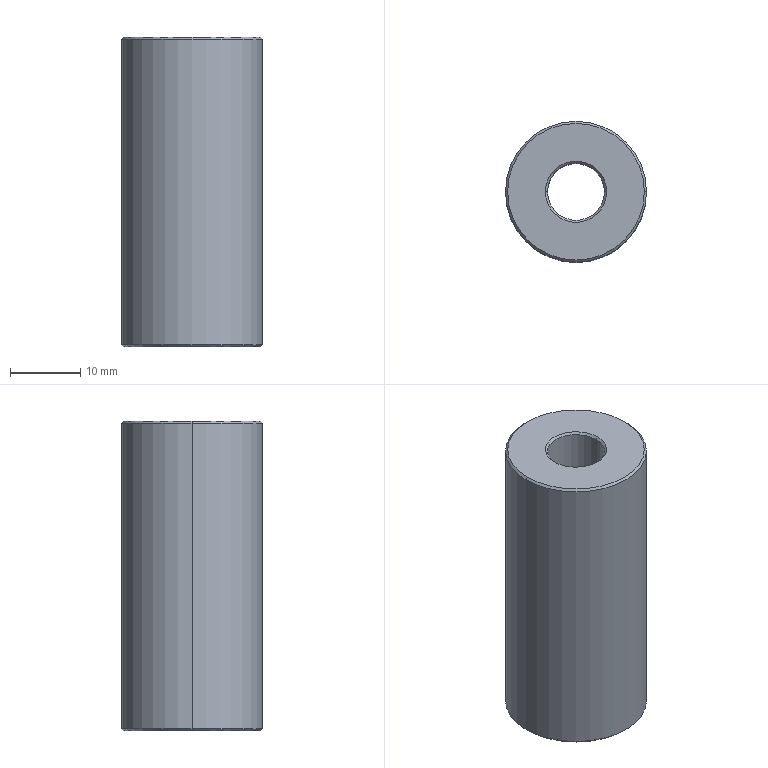Part | SolidWorks | features BaseBody 1 | 1 solid | 14 faces | box 20 x 20 x 44 mm | volume 11548 mm3 | cone 8 | cylinder 4 | plane 2 | commonest cylinder face diameters 8.1 x2 20 x2
STEP:
#1=CARTESIAN_POINT('',(-10.,0.,21.7));
#2=VERTEX_POINT('',#1);
#3=CARTESIAN_POINT('',(10.,0.,21.7));
#4=VERTEX_POINT('',#3);
#5=CARTESIAN_POINT('',(0.,0.,21.7));
#6=DIRECTION('',(0.,0.,-1.));
#7=DIRECTION('',(-1.,0.,0.));
#8=AXIS2_PLACEMENT_3D('',#5,#6,#7);
#9=CIRCLE('',#8,10.);
#10=EDGE_CURVE('',#2,#4,#9,.T.);
#11=ORIENTED_EDGE('',*,*,#10,.T.);
#12=CARTESIAN_POINT('',(10.,0.,-21.7));
#13=VERTEX_POINT('',#12);
#14=CARTESIAN_POINT('',(10.,0.,22.));
#15=DIRECTION('',(0.,0.,-1.));
#16=VECTOR('',#15,1000.);
#17=LINE('',#14,#16);
#18=EDGE_CURVE('',#4,#13,#17,.T.);
#19=ORIENTED_EDGE('',*,*,#18,.T.);
#20=CARTESIAN_POINT('',(-10.,0.,-21.7));
#21=VERTEX_POINT('',#20);
#22=CARTESIAN_POINT('',(0.,0.,-21.7));
#23=DIRECTION('',(0.,0.,1.));
#24=DIRECTION('',(-1.,0.,0.));
#25=AXIS2_PLACEMENT_3D('',#22,#23,#24);
#26=CIRCLE('',#25,10.);
#27=EDGE_CURVE('',#13,#21,#26,.T.);
#28=ORIENTED_EDGE('',*,*,#27,.T.);
#29=CARTESIAN_POINT('',(-10.,0.,22.));
#30=DIRECTION('',(0.,0.,-1.));
#31=VECTOR('',#30,1000.);
#32=LINE('',#29,#31);
#33=EDGE_CURVE('',#2,#21,#32,.T.);
#34=ORIENTED_EDGE('',*,*,#33,.F.);
#35=EDGE_LOOP('',(#11,#19,#28,#34));
#36=FACE_OUTER_BOUND('',#35,.T.);
#37=CARTESIAN_POINT('',(0.,0.,22.));
#38=DIRECTION('',(0.,0.,-1.));
#39=DIRECTION('',(-1.,0.,0.));
#40=AXIS2_PLACEMENT_3D('',#37,#38,#39);
#41=CYLINDRICAL_SURFACE('',#40,10.);
#42=ADVANCED_FACE('',(#36),#41,.T.);
#43=CARTESIAN_POINT('',(9.7,0.,-22.));
#44=VERTEX_POINT('',#43);
#45=CARTESIAN_POINT('',(-9.7,0.,-22.));
#46=VERTEX_POINT('',#45);
#47=CARTESIAN_POINT('',(0.,0.,-22.));
#48=DIRECTION('',(0.,0.,1.));
#49=DIRECTION('',(1.,0.,0.));
#50=AXIS2_PLACEMENT_3D('',#47,#48,#49);
#51=CIRCLE('',#50,9.7);
#52=EDGE_CURVE('',#44,#46,#51,.T.);
#53=ORIENTED_EDGE('',*,*,#52,.T.);
#54=CARTESIAN_POINT('',(-10.,0.,-21.7));
#55=DIRECTION('',(-0.7071,0.,0.7071));
#56=VECTOR('',#55,1000.);
#57=LINE('',#54,#56);
#58=EDGE_CURVE('',#46,#21,#57,.T.);
#59=ORIENTED_EDGE('',*,*,#58,.T.);
#60=ORIENTED_EDGE('',*,*,#27,.F.);
#61=CARTESIAN_POINT('',(10.,0.,-21.7));
#62=DIRECTION('',(0.7071,0.,0.7071));
#63=VECTOR('',#62,1000.);
#64=LINE('',#61,#63);
#65=EDGE_CURVE('',#44,#13,#64,.T.);
#66=ORIENTED_EDGE('',*,*,#65,.F.);
#67=EDGE_LOOP('',(#53,#59,#60,#66));
#68=FACE_OUTER_BOUND('',#67,.T.);
#69=CARTESIAN_POINT('',(0.,0.,-21.7));
#70=DIRECTION('',(0.,0.,1.));
#71=DIRECTION('',(1.,0.,0.));
#72=AXIS2_PLACEMENT_3D('',#69,#70,#71);
#73=CONICAL_SURFACE('',#72,10.,0.7854);
#74=ADVANCED_FACE('',(#68),#73,.T.);
#75=CARTESIAN_POINT('',(-9.7,0.,22.));
#76=VERTEX_POINT('',#75);
#77=CARTESIAN_POINT('',(9.7,0.,22.));
#78=VERTEX_POINT('',#77);
#79=CARTESIAN_POINT('',(0.,0.,22.));
#80=DIRECTION('',(0.,0.,-1.));
#81=DIRECTION('',(-1.,0.,0.));
#82=AXIS2_PLACEMENT_3D('',#79,#80,#81);
#83=CIRCLE('',#82,9.7);
#84=EDGE_CURVE('',#76,#78,#83,.T.);
#85=ORIENTED_EDGE('',*,*,#84,.T.);
#86=CARTESIAN_POINT('',(10.,0.,21.7));
#87=DIRECTION('',(0.7071,0.,-0.7071));
#88=VECTOR('',#87,1000.);
#89=LINE('',#86,#88);
#90=EDGE_CURVE('',#78,#4,#89,.T.);
#91=ORIENTED_EDGE('',*,*,#90,.T.);
#92=ORIENTED_EDGE('',*,*,#10,.F.);
#93=CARTESIAN_POINT('',(-10.,0.,21.7));
#94=DIRECTION('',(-0.7071,0.,-0.7071));
#95=VECTOR('',#94,1000.);
#96=LINE('',#93,#95);
#97=EDGE_CURVE('',#76,#2,#96,.T.);
#98=ORIENTED_EDGE('',*,*,#97,.F.);
#99=EDGE_LOOP('',(#85,#91,#92,#98));
#100=FACE_OUTER_BOUND('',#99,.T.);
#101=CARTESIAN_POINT('',(0.,0.,21.7));
#102=DIRECTION('',(0.,0.,-1.));
#103=DIRECTION('',(-1.,0.,0.));
#104=AXIS2_PLACEMENT_3D('',#101,#102,#103);
#105=CONICAL_SURFACE('',#104,10.,0.7854);
#106=ADVANCED_FACE('',(#100),#105,.T.);
#107=CARTESIAN_POINT('',(4.05,0.,-21.7));
#108=VERTEX_POINT('',#107);
#109=CARTESIAN_POINT('',(-4.05,0.,-21.7));
#110=VERTEX_POINT('',#109);
#111=CARTESIAN_POINT('',(0.,0.,-21.7));
#112=DIRECTION('',(0.,0.,-1.));
#113=DIRECTION('',(-1.,0.,0.));
#114=AXIS2_PLACEMENT_3D('',#111,#112,#113);
#115=CIRCLE('',#114,4.05);
#116=EDGE_CURVE('',#108,#110,#115,.T.);
#117=ORIENTED_EDGE('',*,*,#116,.F.);
#118=CARTESIAN_POINT('',(4.35,0.,-22.));
#119=VERTEX_POINT('',#118);
#120=CARTESIAN_POINT('',(4.35,0.,-22.));
#121=DIRECTION('',(0.7071,0.,-0.7071));
#122=VECTOR('',#121,1000.);
#123=LINE('',#120,#122);
#124=EDGE_CURVE('',#108,#119,#123,.T.);
#125=ORIENTED_EDGE('',*,*,#124,.T.);
#126=CARTESIAN_POINT('',(-4.35,0.,-22.));
#127=VERTEX_POINT('',#126);
#128=CARTESIAN_POINT('',(0.,0.,-22.));
#129=DIRECTION('',(0.,0.,-1.));
#130=DIRECTION('',(-1.,0.,0.));
#131=AXIS2_PLACEMENT_3D('',#128,#129,#130);
#132=CIRCLE('',#131,4.35);
#133=EDGE_CURVE('',#119,#127,#132,.T.);
#134=ORIENTED_EDGE('',*,*,#133,.T.);
#135=CARTESIAN_POINT('',(-4.35,0.,-22.));
#136=DIRECTION('',(-0.7071,0.,-0.7071));
#137=VECTOR('',#136,1000.);
#138=LINE('',#135,#137);
#139=EDGE_CURVE('',#110,#127,#138,.T.);
#140=ORIENTED_EDGE('',*,*,#139,.F.);
#141=EDGE_LOOP('',(#117,#125,#134,#140));
#142=FACE_OUTER_BOUND('',#141,.T.);
#143=CARTESIAN_POINT('',(0.,0.,-22.));
#144=DIRECTION('',(0.,0.,-1.));
#145=DIRECTION('',(-1.,0.,0.));
#146=AXIS2_PLACEMENT_3D('',#143,#144,#145);
#147=CONICAL_SURFACE('',#146,4.35,0.7854);
#148=ADVANCED_FACE('',(#142),#147,.F.);
#149=CARTESIAN_POINT('',(-4.05,0.,21.7));
#150=VERTEX_POINT('',#149);
#151=CARTESIAN_POINT('',(4.05,0.,21.7));
#152=VERTEX_POINT('',#151);
#153=CARTESIAN_POINT('',(0.,0.,21.7));
#154=DIRECTION('',(0.,0.,1.));
#155=DIRECTION('',(1.,0.,0.));
#156=AXIS2_PLACEMENT_3D('',#153,#154,#155);
#157=CIRCLE('',#156,4.05);
#158=EDGE_CURVE('',#150,#152,#157,.T.);
#159=ORIENTED_EDGE('',*,*,#158,.F.);
#160=CARTESIAN_POINT('',(-4.35,0.,22.));
#161=VERTEX_POINT('',#160);
#162=CARTESIAN_POINT('',(-4.35,0.,22.));
#163=DIRECTION('',(-0.7071,0.,0.7071));
#164=VECTOR('',#163,1000.);
#165=LINE('',#162,#164);
#166=EDGE_CURVE('',#150,#161,#165,.T.);
#167=ORIENTED_EDGE('',*,*,#166,.T.);
#168=CARTESIAN_POINT('',(4.35,0.,22.));
#169=VERTEX_POINT('',#168);
#170=CARTESIAN_POINT('',(0.,0.,22.));
#171=DIRECTION('',(0.,0.,-1.));
#172=DIRECTION('',(1.,0.,0.));
#173=AXIS2_PLACEMENT_3D('',#170,#171,#172);
#174=CIRCLE('',#173,4.35);
#175=EDGE_CURVE('',#169,#161,#174,.T.);
#176=ORIENTED_EDGE('',*,*,#175,.F.);
#177=CARTESIAN_POINT('',(4.35,0.,22.));
#178=DIRECTION('',(0.7071,0.,0.7071));
#179=VECTOR('',#178,1000.);
#180=LINE('',#177,#179);
#181=EDGE_CURVE('',#152,#169,#180,.T.);
#182=ORIENTED_EDGE('',*,*,#181,.F.);
#183=EDGE_LOOP('',(#159,#167,#176,#182));
#184=FACE_OUTER_BOUND('',#183,.T.);
#185=CARTESIAN_POINT('',(0.,0.,22.));
#186=DIRECTION('',(0.,0.,1.));
#187=DIRECTION('',(1.,0.,0.));
#188=AXIS2_PLACEMENT_3D('',#185,#186,#187);
#189=CONICAL_SURFACE('',#188,4.35,0.7854);
#190=ADVANCED_FACE('',(#184),#189,.F.);
#191=ORIENTED_EDGE('',*,*,#158,.T.);
#192=CARTESIAN_POINT('',(4.05,0.,22.));
#193=DIRECTION('',(0.,0.,-1.));
#194=VECTOR('',#193,1000.);
#195=LINE('',#192,#194);
#196=EDGE_CURVE('',#152,#108,#195,.T.);
#197=ORIENTED_EDGE('',*,*,#196,.T.);
#198=ORIENTED_EDGE('',*,*,#116,.T.);
#199=CARTESIAN_POINT('',(-4.05,0.,22.));
#200=DIRECTION('',(0.,0.,-1.));
#201=VECTOR('',#200,1000.);
#202=LINE('',#199,#201);
#203=EDGE_CURVE('',#150,#110,#202,.T.);
#204=ORIENTED_EDGE('',*,*,#203,.F.);
#205=EDGE_LOOP('',(#191,#197,#198,#204));
#206=FACE_OUTER_BOUND('',#205,.T.);
#207=CARTESIAN_POINT('',(0.,0.,22.));
#208=DIRECTION('',(0.,0.,-1.));
#209=DIRECTION('',(-1.,0.,0.));
#210=AXIS2_PLACEMENT_3D('',#207,#208,#209);
#211=CYLINDRICAL_SURFACE('',#210,4.05);
#212=ADVANCED_FACE('',(#206),#211,.F.);
#213=ORIENTED_EDGE('',*,*,#18,.F.);
#214=CARTESIAN_POINT('',(0.,0.,21.7));
#215=DIRECTION('',(0.,0.,-1.));
#216=DIRECTION('',(-1.,0.,0.));
#217=AXIS2_PLACEMENT_3D('',#214,#215,#216);
#218=CIRCLE('',#217,10.);
#219=EDGE_CURVE('',#4,#2,#218,.T.);
#220=ORIENTED_EDGE('',*,*,#219,.T.);
#221=ORIENTED_EDGE('',*,*,#33,.T.);
#222=CARTESIAN_POINT('',(0.,0.,-21.7));
#223=DIRECTION('',(0.,0.,1.));
#224=DIRECTION('',(-1.,0.,0.));
#225=AXIS2_PLACEMENT_3D('',#222,#223,#224);
#226=CIRCLE('',#225,10.);
#227=EDGE_CURVE('',#21,#13,#226,.T.);
#228=ORIENTED_EDGE('',*,*,#227,.T.);
#229=EDGE_LOOP('',(#213,#220,#221,#228));
#230=FACE_OUTER_BOUND('',#229,.T.);
#231=CARTESIAN_POINT('',(0.,0.,22.));
#232=DIRECTION('',(0.,0.,-1.));
#233=DIRECTION('',(-1.,0.,0.));
#234=AXIS2_PLACEMENT_3D('',#231,#232,#233);
#235=CYLINDRICAL_SURFACE('',#234,10.);
#236=ADVANCED_FACE('',(#230),#235,.T.);
#237=ORIENTED_EDGE('',*,*,#58,.F.);
#238=CARTESIAN_POINT('',(0.,0.,-22.));
#239=DIRECTION('',(0.,0.,1.));
#240=DIRECTION('',(1.,0.,0.));
#241=AXIS2_PLACEMENT_3D('',#238,#239,#240);
#242=CIRCLE('',#241,9.7);
#243=EDGE_CURVE('',#46,#44,#242,.T.);
#244=ORIENTED_EDGE('',*,*,#243,.T.);
#245=ORIENTED_EDGE('',*,*,#65,.T.);
#246=ORIENTED_EDGE('',*,*,#227,.F.);
#247=EDGE_LOOP('',(#237,#244,#245,#246));
#248=FACE_OUTER_BOUND('',#247,.T.);
#249=CARTESIAN_POINT('',(0.,0.,-21.7));
#250=DIRECTION('',(0.,0.,1.));
#251=DIRECTION('',(1.,0.,0.));
#252=AXIS2_PLACEMENT_3D('',#249,#250,#251);
#253=CONICAL_SURFACE('',#252,10.,0.7854);
#254=ADVANCED_FACE('',(#248),#253,.T.);
#255=ORIENTED_EDGE('',*,*,#90,.F.);
#256=CARTESIAN_POINT('',(0.,0.,22.));
#257=DIRECTION('',(0.,0.,-1.));
#258=DIRECTION('',(-1.,0.,0.));
#259=AXIS2_PLACEMENT_3D('',#256,#257,#258);
#260=CIRCLE('',#259,9.7);
#261=EDGE_CURVE('',#78,#76,#260,.T.);
#262=ORIENTED_EDGE('',*,*,#261,.T.);
#263=ORIENTED_EDGE('',*,*,#97,.T.);
#264=ORIENTED_EDGE('',*,*,#219,.F.);
#265=EDGE_LOOP('',(#255,#262,#263,#264));
#266=FACE_OUTER_BOUND('',#265,.T.);
#267=CARTESIAN_POINT('',(0.,0.,21.7));
#268=DIRECTION('',(0.,0.,-1.));
#269=DIRECTION('',(-1.,0.,0.));
#270=AXIS2_PLACEMENT_3D('',#267,#268,#269);
#271=CONICAL_SURFACE('',#270,10.,0.7854);
#272=ADVANCED_FACE('',(#266),#271,.T.);
#273=CARTESIAN_POINT('',(0.,0.,-22.));
#274=DIRECTION('',(0.,0.,-1.));
#275=DIRECTION('',(-1.,0.,0.));
#276=AXIS2_PLACEMENT_3D('',#273,#274,#275);
#277=CIRCLE('',#276,4.35);
#278=EDGE_CURVE('',#127,#119,#277,.T.);
#279=ORIENTED_EDGE('',*,*,#278,.F.);
#280=ORIENTED_EDGE('',*,*,#133,.F.);
#281=EDGE_LOOP('',(#279,#280));
#282=FACE_BOUND('',#281,.T.);
#283=ORIENTED_EDGE('',*,*,#52,.F.);
#284=ORIENTED_EDGE('',*,*,#243,.F.);
#285=EDGE_LOOP('',(#283,#284));
#286=FACE_OUTER_BOUND('',#285,.T.);
#287=CARTESIAN_POINT('',(0.,0.,-22.));
#288=DIRECTION('',(0.,0.,1.));
#289=DIRECTION('',(1.,0.,0.));
#290=AXIS2_PLACEMENT_3D('',#287,#288,#289);
#291=PLANE('',#290);
#292=ADVANCED_FACE('',(#282,#286),#291,.F.);
#293=ORIENTED_EDGE('',*,*,#84,.F.);
#294=ORIENTED_EDGE('',*,*,#261,.F.);
#295=EDGE_LOOP('',(#293,#294));
#296=FACE_OUTER_BOUND('',#295,.T.);
#297=ORIENTED_EDGE('',*,*,#175,.T.);
#298=CARTESIAN_POINT('',(0.,0.,22.));
#299=DIRECTION('',(0.,0.,-1.));
#300=DIRECTION('',(1.,0.,0.));
#301=AXIS2_PLACEMENT_3D('',#298,#299,#300);
#302=CIRCLE('',#301,4.35);
#303=EDGE_CURVE('',#161,#169,#302,.T.);
#304=ORIENTED_EDGE('',*,*,#303,.T.);
#305=EDGE_LOOP('',(#297,#304));
#306=FACE_BOUND('',#305,.T.);
#307=CARTESIAN_POINT('',(0.,0.,22.));
#308=DIRECTION('',(0.,0.,1.));
#309=DIRECTION('',(1.,0.,0.));
#310=AXIS2_PLACEMENT_3D('',#307,#308,#309);
#311=PLANE('',#310);
#312=ADVANCED_FACE('',(#296,#306),#311,.T.);
#313=ORIENTED_EDGE('',*,*,#124,.F.);
#314=CARTESIAN_POINT('',(0.,0.,-21.7));
#315=DIRECTION('',(0.,0.,-1.));
#316=DIRECTION('',(-1.,0.,0.));
#317=AXIS2_PLACEMENT_3D('',#314,#315,#316);
#318=CIRCLE('',#317,4.05);
#319=EDGE_CURVE('',#110,#108,#318,.T.);
#320=ORIENTED_EDGE('',*,*,#319,.F.);
#321=ORIENTED_EDGE('',*,*,#139,.T.);
#322=ORIENTED_EDGE('',*,*,#278,.T.);
#323=EDGE_LOOP('',(#313,#320,#321,#322));
#324=FACE_OUTER_BOUND('',#323,.T.);
#325=CARTESIAN_POINT('',(0.,0.,-22.));
#326=DIRECTION('',(0.,0.,-1.));
#327=DIRECTION('',(-1.,0.,0.));
#328=AXIS2_PLACEMENT_3D('',#325,#326,#327);
#329=CONICAL_SURFACE('',#328,4.35,0.7854);
#330=ADVANCED_FACE('',(#324),#329,.F.);
#331=ORIENTED_EDGE('',*,*,#166,.F.);
#332=CARTESIAN_POINT('',(0.,0.,21.7));
#333=DIRECTION('',(0.,0.,1.));
#334=DIRECTION('',(1.,0.,0.));
#335=AXIS2_PLACEMENT_3D('',#332,#333,#334);
#336=CIRCLE('',#335,4.05);
#337=EDGE_CURVE('',#152,#150,#336,.T.);
#338=ORIENTED_EDGE('',*,*,#337,.F.);
#339=ORIENTED_EDGE('',*,*,#181,.T.);
#340=ORIENTED_EDGE('',*,*,#303,.F.);
#341=EDGE_LOOP('',(#331,#338,#339,#340));
#342=FACE_OUTER_BOUND('',#341,.T.);
#343=CARTESIAN_POINT('',(0.,0.,22.));
#344=DIRECTION('',(0.,0.,1.));
#345=DIRECTION('',(1.,0.,0.));
#346=AXIS2_PLACEMENT_3D('',#343,#344,#345);
#347=CONICAL_SURFACE('',#346,4.35,0.7854);
#348=ADVANCED_FACE('',(#342),#347,.F.);
#349=ORIENTED_EDGE('',*,*,#196,.F.);
#350=ORIENTED_EDGE('',*,*,#337,.T.);
#351=ORIENTED_EDGE('',*,*,#203,.T.);
#352=ORIENTED_EDGE('',*,*,#319,.T.);
#353=EDGE_LOOP('',(#349,#350,#351,#352));
#354=FACE_OUTER_BOUND('',#353,.T.);
#355=CARTESIAN_POINT('',(0.,0.,22.));
#356=DIRECTION('',(0.,0.,-1.));
#357=DIRECTION('',(-1.,0.,0.));
#358=AXIS2_PLACEMENT_3D('',#355,#356,#357);
#359=CYLINDRICAL_SURFACE('',#358,4.05);
#360=ADVANCED_FACE('',(#354),#359,.F.);
#361=CLOSED_SHELL('',(#42,#74,#106,#148,#190,#212,#236,#254,#272,#292,#312,#330,#348,#360));
#362=MANIFOLD_SOLID_BREP('',#361);
#363=CARTESIAN_POINT('',(0.,0.,0.));
#364=DIRECTION('',(0.,0.,1.));
#365=DIRECTION('',(1.,0.,0.));
#366=AXIS2_PLACEMENT_3D('',#363,#364,#365);
#367=(LENGTH_UNIT()NAMED_UNIT(*)SI_UNIT(.MILLI.,.METRE.));
#368=UNCERTAINTY_MEASURE_WITH_UNIT(LENGTH_MEASURE(0.00001),#367,'','');
#369=(NAMED_UNIT(*)PLANE_ANGLE_UNIT()SI_UNIT($,.RADIAN.));
#370=(NAMED_UNIT(*)SI_UNIT($,.STERADIAN.)SOLID_ANGLE_UNIT());
#371=(GEOMETRIC_REPRESENTATION_CONTEXT(3)GLOBAL_UNCERTAINTY_ASSIGNED_CONTEXT((#368))GLOBAL_UNIT_ASSIGNED_CONTEXT((#367,#369,#370))REPRESENTATION_CONTEXT('',''));
#372=ADVANCED_BREP_SHAPE_REPRESENTATION('',(#362,#366),#371);